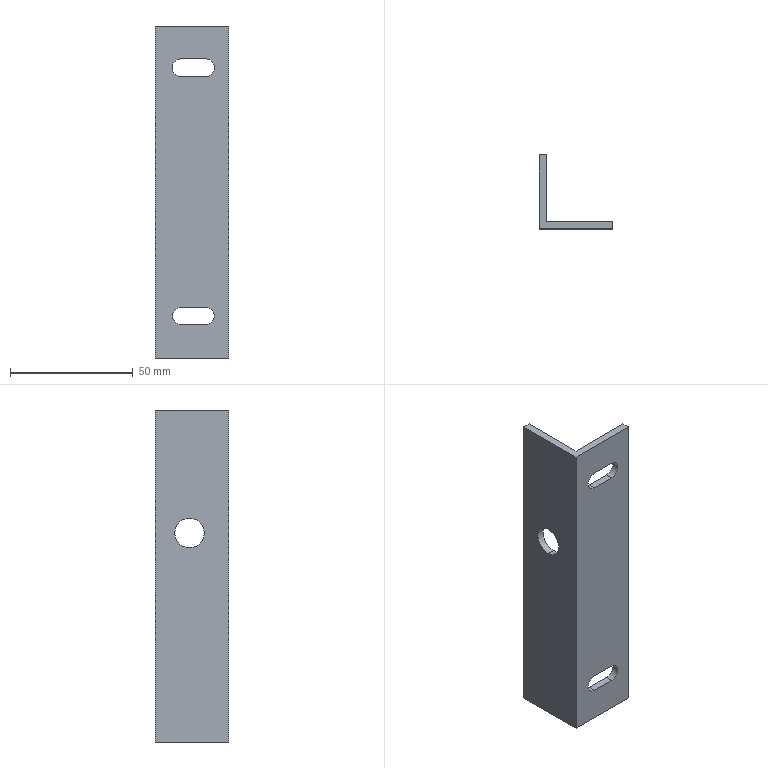Part | SolidWorks | features ICE 2, Extrusion 1 | 1 solid | 18 faces | box 30 x 30 x 135 mm | volume 22072 mm3 | plane 12 | cylinder 6 | commonest cylinder face diameters 7.138 x2 7.334 x2 12 x2
STEP:
#1=CARTESIAN_POINT('',(3.,16.,79.));
#2=VERTEX_POINT('',#1);
#3=CARTESIAN_POINT('',(3.,16.,91.));
#4=VERTEX_POINT('',#3);
#5=CARTESIAN_POINT('',(3.,16.,85.));
#6=DIRECTION('',(-1.,0.,0.));
#7=DIRECTION('',(0.,0.,1.));
#8=AXIS2_PLACEMENT_3D('',#5,#6,#7);
#9=CIRCLE('',#8,6.);
#10=EDGE_CURVE('',#2,#4,#9,.T.);
#11=ORIENTED_EDGE('',*,*,#10,.F.);
#12=CARTESIAN_POINT('',(0.,16.,79.));
#13=VERTEX_POINT('',#12);
#14=CARTESIAN_POINT('',(10.,16.,79.));
#15=DIRECTION('',(-1.,0.,0.));
#16=VECTOR('',#15,1000.);
#17=LINE('',#14,#16);
#18=EDGE_CURVE('',#2,#13,#17,.T.);
#19=ORIENTED_EDGE('',*,*,#18,.T.);
#20=CARTESIAN_POINT('',(0.,16.,91.));
#21=VERTEX_POINT('',#20);
#22=CARTESIAN_POINT('',(0.,16.,85.));
#23=DIRECTION('',(-1.,0.,0.));
#24=DIRECTION('',(0.,0.,1.));
#25=AXIS2_PLACEMENT_3D('',#22,#23,#24);
#26=CIRCLE('',#25,6.);
#27=EDGE_CURVE('',#13,#21,#26,.T.);
#28=ORIENTED_EDGE('',*,*,#27,.T.);
#29=CARTESIAN_POINT('',(10.,16.,91.));
#30=DIRECTION('',(-1.,0.,0.));
#31=VECTOR('',#30,1000.);
#32=LINE('',#29,#31);
#33=EDGE_CURVE('',#4,#21,#32,.T.);
#34=ORIENTED_EDGE('',*,*,#33,.F.);
#35=EDGE_LOOP('',(#11,#19,#28,#34));
#36=FACE_OUTER_BOUND('',#35,.T.);
#37=CARTESIAN_POINT('',(10.,16.,85.));
#38=DIRECTION('',(-1.,0.,0.));
#39=DIRECTION('',(0.,0.,1.));
#40=AXIS2_PLACEMENT_3D('',#37,#38,#39);
#41=CYLINDRICAL_SURFACE('',#40,6.);
#42=ADVANCED_FACE('',(#36),#41,.F.);
#43=CARTESIAN_POINT('',(20.495,0.,114.318));
#44=VERTEX_POINT('',#43);
#45=CARTESIAN_POINT('',(10.659,0.,114.318));
#46=VERTEX_POINT('',#45);
#47=CARTESIAN_POINT('',(0.,0.,114.318));
#48=DIRECTION('',(-1.,0.,0.));
#49=VECTOR('',#48,1000.);
#50=LINE('',#47,#49);
#51=EDGE_CURVE('',#44,#46,#50,.T.);
#52=ORIENTED_EDGE('',*,*,#51,.T.);
#53=CARTESIAN_POINT('',(10.659,0.,121.651));
#54=VERTEX_POINT('',#53);
#55=CARTESIAN_POINT('',(10.659,0.,117.985));
#56=DIRECTION('',(0.,1.,0.));
#57=DIRECTION('',(0.,0.,1.));
#58=AXIS2_PLACEMENT_3D('',#55,#56,#57);
#59=CIRCLE('',#58,3.667);
#60=EDGE_CURVE('',#46,#54,#59,.T.);
#61=ORIENTED_EDGE('',*,*,#60,.T.);
#62=CARTESIAN_POINT('',(20.495,0.,121.651));
#63=VERTEX_POINT('',#62);
#64=CARTESIAN_POINT('',(0.,0.,121.651));
#65=DIRECTION('',(1.,0.,0.));
#66=VECTOR('',#65,1000.);
#67=LINE('',#64,#66);
#68=EDGE_CURVE('',#54,#63,#67,.T.);
#69=ORIENTED_EDGE('',*,*,#68,.T.);
#70=CARTESIAN_POINT('',(20.495,0.,117.985));
#71=DIRECTION('',(0.,1.,0.));
#72=DIRECTION('',(0.,0.,1.));
#73=AXIS2_PLACEMENT_3D('',#70,#71,#72);
#74=CIRCLE('',#73,3.667);
#75=EDGE_CURVE('',#63,#44,#74,.T.);
#76=ORIENTED_EDGE('',*,*,#75,.T.);
#77=EDGE_LOOP('',(#52,#61,#69,#76));
#78=FACE_BOUND('',#77,.T.);
#79=CARTESIAN_POINT('',(20.495,0.,13.532));
#80=VERTEX_POINT('',#79);
#81=CARTESIAN_POINT('',(10.659,0.,13.532));
#82=VERTEX_POINT('',#81);
#83=CARTESIAN_POINT('',(0.,0.,13.532));
#84=DIRECTION('',(-1.,0.,0.));
#85=VECTOR('',#84,1000.);
#86=LINE('',#83,#85);
#87=EDGE_CURVE('',#80,#82,#86,.T.);
#88=ORIENTED_EDGE('',*,*,#87,.T.);
#89=CARTESIAN_POINT('',(10.659,0.,20.67));
#90=VERTEX_POINT('',#89);
#91=CARTESIAN_POINT('',(10.659,0.,17.101));
#92=DIRECTION('',(0.,1.,0.));
#93=DIRECTION('',(0.,0.,1.));
#94=AXIS2_PLACEMENT_3D('',#91,#92,#93);
#95=CIRCLE('',#94,3.569);
#96=EDGE_CURVE('',#82,#90,#95,.T.);
#97=ORIENTED_EDGE('',*,*,#96,.T.);
#98=CARTESIAN_POINT('',(20.495,0.,20.67));
#99=VERTEX_POINT('',#98);
#100=CARTESIAN_POINT('',(0.,0.,20.67));
#101=DIRECTION('',(1.,0.,0.));
#102=VECTOR('',#101,1000.);
#103=LINE('',#100,#102);
#104=EDGE_CURVE('',#90,#99,#103,.T.);
#105=ORIENTED_EDGE('',*,*,#104,.T.);
#106=CARTESIAN_POINT('',(20.495,0.,17.101));
#107=DIRECTION('',(0.,1.,0.));
#108=DIRECTION('',(0.,0.,1.));
#109=AXIS2_PLACEMENT_3D('',#106,#107,#108);
#110=CIRCLE('',#109,3.569);
#111=EDGE_CURVE('',#99,#80,#110,.T.);
#112=ORIENTED_EDGE('',*,*,#111,.T.);
#113=EDGE_LOOP('',(#88,#97,#105,#112));
#114=FACE_BOUND('',#113,.T.);
#115=CARTESIAN_POINT('',(0.,0.,0.));
#116=VERTEX_POINT('',#115);
#117=CARTESIAN_POINT('',(30.,0.,0.));
#118=VERTEX_POINT('',#117);
#119=CARTESIAN_POINT('',(0.,0.,0.));
#120=DIRECTION('',(1.,0.,0.));
#121=VECTOR('',#120,1000.);
#122=LINE('',#119,#121);
#123=EDGE_CURVE('',#116,#118,#122,.T.);
#124=ORIENTED_EDGE('',*,*,#123,.T.);
#125=CARTESIAN_POINT('',(30.,0.,135.));
#126=VERTEX_POINT('',#125);
#127=CARTESIAN_POINT('',(30.,0.,135.));
#128=DIRECTION('',(0.,0.,-1.));
#129=VECTOR('',#128,1000.);
#130=LINE('',#127,#129);
#131=EDGE_CURVE('',#126,#118,#130,.T.);
#132=ORIENTED_EDGE('',*,*,#131,.F.);
#133=CARTESIAN_POINT('',(0.,0.,135.));
#134=VERTEX_POINT('',#133);
#135=CARTESIAN_POINT('',(0.,0.,135.));
#136=DIRECTION('',(1.,0.,0.));
#137=VECTOR('',#136,1000.);
#138=LINE('',#135,#137);
#139=EDGE_CURVE('',#134,#126,#138,.T.);
#140=ORIENTED_EDGE('',*,*,#139,.F.);
#141=CARTESIAN_POINT('',(0.,0.,135.));
#142=DIRECTION('',(0.,0.,-1.));
#143=VECTOR('',#142,1000.);
#144=LINE('',#141,#143);
#145=EDGE_CURVE('',#134,#116,#144,.T.);
#146=ORIENTED_EDGE('',*,*,#145,.T.);
#147=EDGE_LOOP('',(#124,#132,#140,#146));
#148=FACE_OUTER_BOUND('',#147,.T.);
#149=CARTESIAN_POINT('',(0.,0.,135.));
#150=DIRECTION('',(0.,1.,0.));
#151=DIRECTION('',(0.,0.,1.));
#152=AXIS2_PLACEMENT_3D('',#149,#150,#151);
#153=PLANE('',#152);
#154=ADVANCED_FACE('',(#78,#114,#148),#153,.F.);
#155=CARTESIAN_POINT('',(30.,3.,0.));
#156=VERTEX_POINT('',#155);
#157=CARTESIAN_POINT('',(30.,3.,0.));
#158=DIRECTION('',(0.,1.,0.));
#159=VECTOR('',#158,1000.);
#160=LINE('',#157,#159);
#161=EDGE_CURVE('',#118,#156,#160,.T.);
#162=ORIENTED_EDGE('',*,*,#161,.T.);
#163=CARTESIAN_POINT('',(30.,3.,135.));
#164=VERTEX_POINT('',#163);
#165=CARTESIAN_POINT('',(30.,3.,135.));
#166=DIRECTION('',(0.,0.,-1.));
#167=VECTOR('',#166,1000.);
#168=LINE('',#165,#167);
#169=EDGE_CURVE('',#164,#156,#168,.T.);
#170=ORIENTED_EDGE('',*,*,#169,.F.);
#171=CARTESIAN_POINT('',(30.,3.,135.));
#172=DIRECTION('',(0.,1.,0.));
#173=VECTOR('',#172,1000.);
#174=LINE('',#171,#173);
#175=EDGE_CURVE('',#126,#164,#174,.T.);
#176=ORIENTED_EDGE('',*,*,#175,.F.);
#177=ORIENTED_EDGE('',*,*,#131,.T.);
#178=EDGE_LOOP('',(#162,#170,#176,#177));
#179=FACE_OUTER_BOUND('',#178,.T.);
#180=CARTESIAN_POINT('',(30.,3.,135.));
#181=DIRECTION('',(-1.,0.,0.));
#182=DIRECTION('',(0.,0.,1.));
#183=AXIS2_PLACEMENT_3D('',#180,#181,#182);
#184=PLANE('',#183);
#185=ADVANCED_FACE('',(#179),#184,.F.);
#186=CARTESIAN_POINT('',(10.659,3.,121.651));
#187=VERTEX_POINT('',#186);
#188=CARTESIAN_POINT('',(20.495,3.,121.651));
#189=VERTEX_POINT('',#188);
#190=CARTESIAN_POINT('',(10.659,3.,121.651));
#191=DIRECTION('',(1.,0.,0.));
#192=VECTOR('',#191,1000.);
#193=LINE('',#190,#192);
#194=EDGE_CURVE('',#187,#189,#193,.T.);
#195=ORIENTED_EDGE('',*,*,#194,.F.);
#196=CARTESIAN_POINT('',(10.659,3.,114.318));
#197=VERTEX_POINT('',#196);
#198=CARTESIAN_POINT('',(10.659,3.,117.985));
#199=DIRECTION('',(0.,1.,0.));
#200=DIRECTION('',(0.,0.,1.));
#201=AXIS2_PLACEMENT_3D('',#198,#199,#200);
#202=CIRCLE('',#201,3.667);
#203=EDGE_CURVE('',#197,#187,#202,.T.);
#204=ORIENTED_EDGE('',*,*,#203,.F.);
#205=CARTESIAN_POINT('',(20.495,3.,114.318));
#206=VERTEX_POINT('',#205);
#207=CARTESIAN_POINT('',(10.659,3.,114.318));
#208=DIRECTION('',(-1.,0.,0.));
#209=VECTOR('',#208,1000.);
#210=LINE('',#207,#209);
#211=EDGE_CURVE('',#206,#197,#210,.T.);
#212=ORIENTED_EDGE('',*,*,#211,.F.);
#213=CARTESIAN_POINT('',(20.495,3.,117.985));
#214=DIRECTION('',(0.,1.,0.));
#215=DIRECTION('',(0.,0.,1.));
#216=AXIS2_PLACEMENT_3D('',#213,#214,#215);
#217=CIRCLE('',#216,3.667);
#218=EDGE_CURVE('',#189,#206,#217,.T.);
#219=ORIENTED_EDGE('',*,*,#218,.F.);
#220=EDGE_LOOP('',(#195,#204,#212,#219));
#221=FACE_BOUND('',#220,.T.);
#222=CARTESIAN_POINT('',(10.659,3.,20.67));
#223=VERTEX_POINT('',#222);
#224=CARTESIAN_POINT('',(20.495,3.,20.67));
#225=VERTEX_POINT('',#224);
#226=CARTESIAN_POINT('',(10.659,3.,20.67));
#227=DIRECTION('',(1.,0.,0.));
#228=VECTOR('',#227,1000.);
#229=LINE('',#226,#228);
#230=EDGE_CURVE('',#223,#225,#229,.T.);
#231=ORIENTED_EDGE('',*,*,#230,.F.);
#232=CARTESIAN_POINT('',(10.659,3.,13.532));
#233=VERTEX_POINT('',#232);
#234=CARTESIAN_POINT('',(10.659,3.,17.101));
#235=DIRECTION('',(0.,1.,0.));
#236=DIRECTION('',(0.,0.,1.));
#237=AXIS2_PLACEMENT_3D('',#234,#235,#236);
#238=CIRCLE('',#237,3.569);
#239=EDGE_CURVE('',#233,#223,#238,.T.);
#240=ORIENTED_EDGE('',*,*,#239,.F.);
#241=CARTESIAN_POINT('',(20.495,3.,13.532));
#242=VERTEX_POINT('',#241);
#243=CARTESIAN_POINT('',(10.659,3.,13.532));
#244=DIRECTION('',(-1.,0.,0.));
#245=VECTOR('',#244,1000.);
#246=LINE('',#243,#245);
#247=EDGE_CURVE('',#242,#233,#246,.T.);
#248=ORIENTED_EDGE('',*,*,#247,.F.);
#249=CARTESIAN_POINT('',(20.495,3.,17.101));
#250=DIRECTION('',(0.,1.,0.));
#251=DIRECTION('',(0.,0.,1.));
#252=AXIS2_PLACEMENT_3D('',#249,#250,#251);
#253=CIRCLE('',#252,3.569);
#254=EDGE_CURVE('',#225,#242,#253,.T.);
#255=ORIENTED_EDGE('',*,*,#254,.F.);
#256=EDGE_LOOP('',(#231,#240,#248,#255));
#257=FACE_BOUND('',#256,.T.);
#258=CARTESIAN_POINT('',(3.,3.,0.));
#259=VERTEX_POINT('',#258);
#260=CARTESIAN_POINT('',(3.,3.,0.));
#261=DIRECTION('',(-1.,0.,0.));
#262=VECTOR('',#261,1000.);
#263=LINE('',#260,#262);
#264=EDGE_CURVE('',#156,#259,#263,.T.);
#265=ORIENTED_EDGE('',*,*,#264,.T.);
#266=CARTESIAN_POINT('',(3.,3.,135.));
#267=VERTEX_POINT('',#266);
#268=CARTESIAN_POINT('',(3.,3.,135.));
#269=DIRECTION('',(0.,0.,-1.));
#270=VECTOR('',#269,1000.);
#271=LINE('',#268,#270);
#272=EDGE_CURVE('',#267,#259,#271,.T.);
#273=ORIENTED_EDGE('',*,*,#272,.F.);
#274=CARTESIAN_POINT('',(3.,3.,135.));
#275=DIRECTION('',(-1.,0.,0.));
#276=VECTOR('',#275,1000.);
#277=LINE('',#274,#276);
#278=EDGE_CURVE('',#164,#267,#277,.T.);
#279=ORIENTED_EDGE('',*,*,#278,.F.);
#280=ORIENTED_EDGE('',*,*,#169,.T.);
#281=EDGE_LOOP('',(#265,#273,#279,#280));
#282=FACE_OUTER_BOUND('',#281,.T.);
#283=CARTESIAN_POINT('',(3.,3.,135.));
#284=DIRECTION('',(0.,-1.,0.));
#285=DIRECTION('',(0.,0.,-1.));
#286=AXIS2_PLACEMENT_3D('',#283,#284,#285);
#287=PLANE('',#286);
#288=ADVANCED_FACE('',(#221,#257,#282),#287,.F.);
#289=CARTESIAN_POINT('',(3.,16.,85.));
#290=DIRECTION('',(-1.,0.,0.));
#291=DIRECTION('',(0.,0.,1.));
#292=AXIS2_PLACEMENT_3D('',#289,#290,#291);
#293=CIRCLE('',#292,6.);
#294=EDGE_CURVE('',#4,#2,#293,.T.);
#295=ORIENTED_EDGE('',*,*,#294,.T.);
#296=ORIENTED_EDGE('',*,*,#10,.T.);
#297=EDGE_LOOP('',(#295,#296));
#298=FACE_BOUND('',#297,.T.);
#299=CARTESIAN_POINT('',(3.,30.,0.));
#300=VERTEX_POINT('',#299);
#301=CARTESIAN_POINT('',(3.,3.,0.));
#302=DIRECTION('',(0.,1.,0.));
#303=VECTOR('',#302,1000.);
#304=LINE('',#301,#303);
#305=EDGE_CURVE('',#259,#300,#304,.T.);
#306=ORIENTED_EDGE('',*,*,#305,.T.);
#307=CARTESIAN_POINT('',(3.,30.,135.));
#308=VERTEX_POINT('',#307);
#309=CARTESIAN_POINT('',(3.,30.,135.));
#310=DIRECTION('',(0.,0.,-1.));
#311=VECTOR('',#310,1000.);
#312=LINE('',#309,#311);
#313=EDGE_CURVE('',#308,#300,#312,.T.);
#314=ORIENTED_EDGE('',*,*,#313,.F.);
#315=CARTESIAN_POINT('',(3.,3.,135.));
#316=DIRECTION('',(0.,1.,0.));
#317=VECTOR('',#316,1000.);
#318=LINE('',#315,#317);
#319=EDGE_CURVE('',#267,#308,#318,.T.);
#320=ORIENTED_EDGE('',*,*,#319,.F.);
#321=ORIENTED_EDGE('',*,*,#272,.T.);
#322=EDGE_LOOP('',(#306,#314,#320,#321));
#323=FACE_OUTER_BOUND('',#322,.T.);
#324=CARTESIAN_POINT('',(3.,3.,135.));
#325=DIRECTION('',(-1.,0.,0.));
#326=DIRECTION('',(0.,0.,1.));
#327=AXIS2_PLACEMENT_3D('',#324,#325,#326);
#328=PLANE('',#327);
#329=ADVANCED_FACE('',(#298,#323),#328,.F.);
#330=CARTESIAN_POINT('',(0.,30.,0.));
#331=VERTEX_POINT('',#330);
#332=CARTESIAN_POINT('',(0.,30.,0.));
#333=DIRECTION('',(-1.,0.,0.));
#334=VECTOR('',#333,1000.);
#335=LINE('',#332,#334);
#336=EDGE_CURVE('',#300,#331,#335,.T.);
#337=ORIENTED_EDGE('',*,*,#336,.T.);
#338=CARTESIAN_POINT('',(0.,30.,135.));
#339=VERTEX_POINT('',#338);
#340=CARTESIAN_POINT('',(0.,30.,135.));
#341=DIRECTION('',(0.,0.,-1.));
#342=VECTOR('',#341,1000.);
#343=LINE('',#340,#342);
#344=EDGE_CURVE('',#339,#331,#343,.T.);
#345=ORIENTED_EDGE('',*,*,#344,.F.);
#346=CARTESIAN_POINT('',(0.,30.,135.));
#347=DIRECTION('',(-1.,0.,0.));
#348=VECTOR('',#347,1000.);
#349=LINE('',#346,#348);
#350=EDGE_CURVE('',#308,#339,#349,.T.);
#351=ORIENTED_EDGE('',*,*,#350,.F.);
#352=ORIENTED_EDGE('',*,*,#313,.T.);
#353=EDGE_LOOP('',(#337,#345,#351,#352));
#354=FACE_OUTER_BOUND('',#353,.T.);
#355=CARTESIAN_POINT('',(0.,30.,135.));
#356=DIRECTION('',(0.,-1.,0.));
#357=DIRECTION('',(0.,0.,-1.));
#358=AXIS2_PLACEMENT_3D('',#355,#356,#357);
#359=PLANE('',#358);
#360=ADVANCED_FACE('',(#354),#359,.F.);
#361=CARTESIAN_POINT('',(0.,16.,85.));
#362=DIRECTION('',(-1.,0.,0.));
#363=DIRECTION('',(0.,0.,1.));
#364=AXIS2_PLACEMENT_3D('',#361,#362,#363);
#365=CIRCLE('',#364,6.);
#366=EDGE_CURVE('',#21,#13,#365,.T.);
#367=ORIENTED_EDGE('',*,*,#366,.F.);
#368=ORIENTED_EDGE('',*,*,#27,.F.);
#369=EDGE_LOOP('',(#367,#368));
#370=FACE_BOUND('',#369,.T.);
#371=CARTESIAN_POINT('',(0.,0.,0.));
#372=DIRECTION('',(0.,-1.,0.));
#373=VECTOR('',#372,1000.);
#374=LINE('',#371,#373);
#375=EDGE_CURVE('',#331,#116,#374,.T.);
#376=ORIENTED_EDGE('',*,*,#375,.T.);
#377=ORIENTED_EDGE('',*,*,#145,.F.);
#378=CARTESIAN_POINT('',(0.,0.,135.));
#379=DIRECTION('',(0.,-1.,0.));
#380=VECTOR('',#379,1000.);
#381=LINE('',#378,#380);
#382=EDGE_CURVE('',#339,#134,#381,.T.);
#383=ORIENTED_EDGE('',*,*,#382,.F.);
#384=ORIENTED_EDGE('',*,*,#344,.T.);
#385=EDGE_LOOP('',(#376,#377,#383,#384));
#386=FACE_OUTER_BOUND('',#385,.T.);
#387=CARTESIAN_POINT('',(0.,0.,135.));
#388=DIRECTION('',(1.,0.,0.));
#389=DIRECTION('',(0.,0.,-1.));
#390=AXIS2_PLACEMENT_3D('',#387,#388,#389);
#391=PLANE('',#390);
#392=ADVANCED_FACE('',(#370,#386),#391,.F.);
#393=ORIENTED_EDGE('',*,*,#139,.T.);
#394=ORIENTED_EDGE('',*,*,#175,.T.);
#395=ORIENTED_EDGE('',*,*,#278,.T.);
#396=ORIENTED_EDGE('',*,*,#319,.T.);
#397=ORIENTED_EDGE('',*,*,#350,.T.);
#398=ORIENTED_EDGE('',*,*,#382,.T.);
#399=EDGE_LOOP('',(#393,#394,#395,#396,#397,#398));
#400=FACE_OUTER_BOUND('',#399,.T.);
#401=CARTESIAN_POINT('',(0.,0.,135.));
#402=DIRECTION('',(0.,0.,-1.));
#403=DIRECTION('',(-1.,0.,0.));
#404=AXIS2_PLACEMENT_3D('',#401,#402,#403);
#405=PLANE('',#404);
#406=ADVANCED_FACE('',(#400),#405,.F.);
#407=ORIENTED_EDGE('',*,*,#123,.F.);
#408=ORIENTED_EDGE('',*,*,#375,.F.);
#409=ORIENTED_EDGE('',*,*,#336,.F.);
#410=ORIENTED_EDGE('',*,*,#305,.F.);
#411=ORIENTED_EDGE('',*,*,#264,.F.);
#412=ORIENTED_EDGE('',*,*,#161,.F.);
#413=EDGE_LOOP('',(#407,#408,#409,#410,#411,#412));
#414=FACE_OUTER_BOUND('',#413,.T.);
#415=CARTESIAN_POINT('',(0.,0.,0.));
#416=DIRECTION('',(0.,0.,-1.));
#417=DIRECTION('',(-1.,0.,0.));
#418=AXIS2_PLACEMENT_3D('',#415,#416,#417);
#419=PLANE('',#418);
#420=ADVANCED_FACE('',(#414),#419,.T.);
#421=CARTESIAN_POINT('',(10.659,-157.,13.532));
#422=DIRECTION('',(0.,1.,0.));
#423=VECTOR('',#422,1000.);
#424=LINE('',#421,#423);
#425=EDGE_CURVE('',#82,#233,#424,.T.);
#426=ORIENTED_EDGE('',*,*,#425,.T.);
#427=ORIENTED_EDGE('',*,*,#239,.T.);
#428=CARTESIAN_POINT('',(10.659,-157.,20.67));
#429=DIRECTION('',(0.,1.,0.));
#430=VECTOR('',#429,1000.);
#431=LINE('',#428,#430);
#432=EDGE_CURVE('',#90,#223,#431,.T.);
#433=ORIENTED_EDGE('',*,*,#432,.F.);
#434=ORIENTED_EDGE('',*,*,#96,.F.);
#435=EDGE_LOOP('',(#426,#427,#433,#434));
#436=FACE_OUTER_BOUND('',#435,.T.);
#437=CARTESIAN_POINT('',(10.659,-157.,17.101));
#438=DIRECTION('',(0.,1.,0.));
#439=DIRECTION('',(0.,0.,1.));
#440=AXIS2_PLACEMENT_3D('',#437,#438,#439);
#441=CYLINDRICAL_SURFACE('',#440,3.569);
#442=ADVANCED_FACE('',(#436),#441,.F.);
#443=CARTESIAN_POINT('',(20.495,-157.,13.532));
#444=DIRECTION('',(0.,1.,0.));
#445=VECTOR('',#444,1000.);
#446=LINE('',#443,#445);
#447=EDGE_CURVE('',#80,#242,#446,.T.);
#448=ORIENTED_EDGE('',*,*,#447,.T.);
#449=ORIENTED_EDGE('',*,*,#247,.T.);
#450=ORIENTED_EDGE('',*,*,#425,.F.);
#451=ORIENTED_EDGE('',*,*,#87,.F.);
#452=EDGE_LOOP('',(#448,#449,#450,#451));
#453=FACE_OUTER_BOUND('',#452,.T.);
#454=CARTESIAN_POINT('',(10.659,-157.,13.532));
#455=DIRECTION('',(0.,0.,-1.));
#456=DIRECTION('',(-1.,0.,0.));
#457=AXIS2_PLACEMENT_3D('',#454,#455,#456);
#458=PLANE('',#457);
#459=ADVANCED_FACE('',(#453),#458,.F.);
#460=CARTESIAN_POINT('',(20.495,-157.,20.67));
#461=DIRECTION('',(0.,1.,0.));
#462=VECTOR('',#461,1000.);
#463=LINE('',#460,#462);
#464=EDGE_CURVE('',#99,#225,#463,.T.);
#465=ORIENTED_EDGE('',*,*,#464,.T.);
#466=ORIENTED_EDGE('',*,*,#254,.T.);
#467=ORIENTED_EDGE('',*,*,#447,.F.);
#468=ORIENTED_EDGE('',*,*,#111,.F.);
#469=EDGE_LOOP('',(#465,#466,#467,#468));
#470=FACE_OUTER_BOUND('',#469,.T.);
#471=CARTESIAN_POINT('',(20.495,-157.,17.101));
#472=DIRECTION('',(0.,1.,0.));
#473=DIRECTION('',(0.,0.,1.));
#474=AXIS2_PLACEMENT_3D('',#471,#472,#473);
#475=CYLINDRICAL_SURFACE('',#474,3.569);
#476=ADVANCED_FACE('',(#470),#475,.F.);
#477=ORIENTED_EDGE('',*,*,#432,.T.);
#478=ORIENTED_EDGE('',*,*,#230,.T.);
#479=ORIENTED_EDGE('',*,*,#464,.F.);
#480=ORIENTED_EDGE('',*,*,#104,.F.);
#481=EDGE_LOOP('',(#477,#478,#479,#480));
#482=FACE_OUTER_BOUND('',#481,.T.);
#483=CARTESIAN_POINT('',(10.659,-157.,20.67));
#484=DIRECTION('',(0.,0.,1.));
#485=DIRECTION('',(1.,0.,0.));
#486=AXIS2_PLACEMENT_3D('',#483,#484,#485);
#487=PLANE('',#486);
#488=ADVANCED_FACE('',(#482),#487,.F.);
#489=CARTESIAN_POINT('',(10.659,-157.,114.318));
#490=DIRECTION('',(0.,1.,0.));
#491=VECTOR('',#490,1000.);
#492=LINE('',#489,#491);
#493=EDGE_CURVE('',#46,#197,#492,.T.);
#494=ORIENTED_EDGE('',*,*,#493,.T.);
#495=ORIENTED_EDGE('',*,*,#203,.T.);
#496=CARTESIAN_POINT('',(10.659,-157.,121.651));
#497=DIRECTION('',(0.,1.,0.));
#498=VECTOR('',#497,1000.);
#499=LINE('',#496,#498);
#500=EDGE_CURVE('',#54,#187,#499,.T.);
#501=ORIENTED_EDGE('',*,*,#500,.F.);
#502=ORIENTED_EDGE('',*,*,#60,.F.);
#503=EDGE_LOOP('',(#494,#495,#501,#502));
#504=FACE_OUTER_BOUND('',#503,.T.);
#505=CARTESIAN_POINT('',(10.659,-157.,117.985));
#506=DIRECTION('',(0.,1.,0.));
#507=DIRECTION('',(0.,0.,1.));
#508=AXIS2_PLACEMENT_3D('',#505,#506,#507);
#509=CYLINDRICAL_SURFACE('',#508,3.667);
#510=ADVANCED_FACE('',(#504),#509,.F.);
#511=CARTESIAN_POINT('',(20.495,-157.,114.318));
#512=DIRECTION('',(0.,1.,0.));
#513=VECTOR('',#512,1000.);
#514=LINE('',#511,#513);
#515=EDGE_CURVE('',#44,#206,#514,.T.);
#516=ORIENTED_EDGE('',*,*,#515,.T.);
#517=ORIENTED_EDGE('',*,*,#211,.T.);
#518=ORIENTED_EDGE('',*,*,#493,.F.);
#519=ORIENTED_EDGE('',*,*,#51,.F.);
#520=EDGE_LOOP('',(#516,#517,#518,#519));
#521=FACE_OUTER_BOUND('',#520,.T.);
#522=CARTESIAN_POINT('',(10.659,-157.,114.318));
#523=DIRECTION('',(0.,0.,-1.));
#524=DIRECTION('',(-1.,0.,0.));
#525=AXIS2_PLACEMENT_3D('',#522,#523,#524);
#526=PLANE('',#525);
#527=ADVANCED_FACE('',(#521),#526,.F.);
#528=CARTESIAN_POINT('',(20.495,-157.,121.651));
#529=DIRECTION('',(0.,1.,0.));
#530=VECTOR('',#529,1000.);
#531=LINE('',#528,#530);
#532=EDGE_CURVE('',#63,#189,#531,.T.);
#533=ORIENTED_EDGE('',*,*,#532,.T.);
#534=ORIENTED_EDGE('',*,*,#218,.T.);
#535=ORIENTED_EDGE('',*,*,#515,.F.);
#536=ORIENTED_EDGE('',*,*,#75,.F.);
#537=EDGE_LOOP('',(#533,#534,#535,#536));
#538=FACE_OUTER_BOUND('',#537,.T.);
#539=CARTESIAN_POINT('',(20.495,-157.,117.985));
#540=DIRECTION('',(0.,1.,0.));
#541=DIRECTION('',(0.,0.,1.));
#542=AXIS2_PLACEMENT_3D('',#539,#540,#541);
#543=CYLINDRICAL_SURFACE('',#542,3.667);
#544=ADVANCED_FACE('',(#538),#543,.F.);
#545=ORIENTED_EDGE('',*,*,#500,.T.);
#546=ORIENTED_EDGE('',*,*,#194,.T.);
#547=ORIENTED_EDGE('',*,*,#532,.F.);
#548=ORIENTED_EDGE('',*,*,#68,.F.);
#549=EDGE_LOOP('',(#545,#546,#547,#548));
#550=FACE_OUTER_BOUND('',#549,.T.);
#551=CARTESIAN_POINT('',(10.659,-157.,121.651));
#552=DIRECTION('',(0.,0.,1.));
#553=DIRECTION('',(1.,0.,0.));
#554=AXIS2_PLACEMENT_3D('',#551,#552,#553);
#555=PLANE('',#554);
#556=ADVANCED_FACE('',(#550),#555,.F.);
#557=ORIENTED_EDGE('',*,*,#18,.F.);
#558=ORIENTED_EDGE('',*,*,#294,.F.);
#559=ORIENTED_EDGE('',*,*,#33,.T.);
#560=ORIENTED_EDGE('',*,*,#366,.T.);
#561=EDGE_LOOP('',(#557,#558,#559,#560));
#562=FACE_OUTER_BOUND('',#561,.T.);
#563=CARTESIAN_POINT('',(10.,16.,85.));
#564=DIRECTION('',(-1.,0.,0.));
#565=DIRECTION('',(0.,0.,1.));
#566=AXIS2_PLACEMENT_3D('',#563,#564,#565);
#567=CYLINDRICAL_SURFACE('',#566,6.);
#568=ADVANCED_FACE('',(#562),#567,.F.);
#569=CLOSED_SHELL('',(#42,#154,#185,#288,#329,#360,#392,#406,#420,#442,#459,#476,#488,#510,#527,#544,#556,#568));
#570=MANIFOLD_SOLID_BREP('',#569);
#571=CARTESIAN_POINT('',(0.,0.,0.));
#572=DIRECTION('',(0.,0.,1.));
#573=DIRECTION('',(1.,0.,0.));
#574=AXIS2_PLACEMENT_3D('',#571,#572,#573);
#575=(LENGTH_UNIT()NAMED_UNIT(*)SI_UNIT(.MILLI.,.METRE.));
#576=UNCERTAINTY_MEASURE_WITH_UNIT(LENGTH_MEASURE(0.00001),#575,'','');
#577=(NAMED_UNIT(*)PLANE_ANGLE_UNIT()SI_UNIT($,.RADIAN.));
#578=(NAMED_UNIT(*)SI_UNIT($,.STERADIAN.)SOLID_ANGLE_UNIT());
#579=(GEOMETRIC_REPRESENTATION_CONTEXT(3)GLOBAL_UNCERTAINTY_ASSIGNED_CONTEXT((#576))GLOBAL_UNIT_ASSIGNED_CONTEXT((#575,#577,#578))REPRESENTATION_CONTEXT('',''));
#580=ADVANCED_BREP_SHAPE_REPRESENTATION('',(#570,#574),#579);